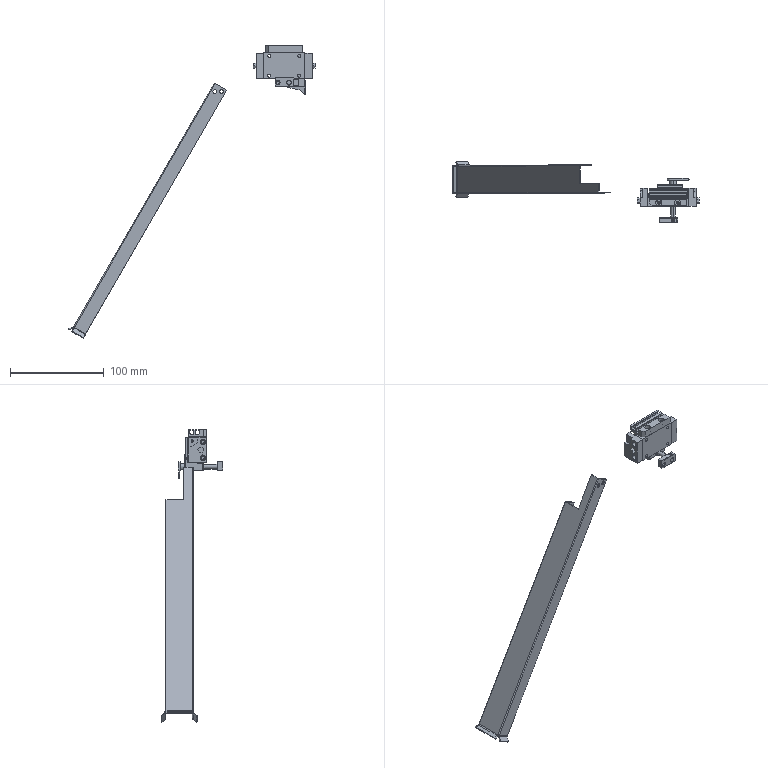Part | NX | 12 solids | 408 faces | box 262.673 x 65.539 x 312.186 mm | volume 55533 mm3 | plane 223 | cylinder 140 | cone 43 | torus 2 | commonest cylinder face diameters 2.5 x32 6 x14 3.2 x12 3.3 x10 3.5 x8 4 x8